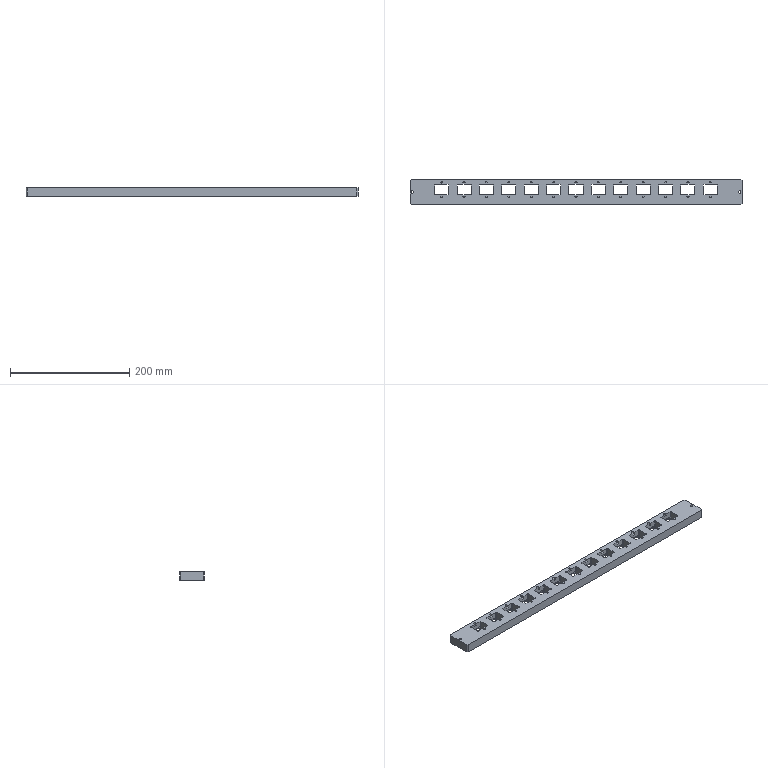NC program | NX | posted with a generic post | part box 556 x 41 x 15 mm
Lines 51164 to 52182 of 52182:
(PLANAR_MILL_COPY , TOOL : D6A45)
N102320 T07 M6
N102322 G54
N102324 G17 G0 G90 X-274.55 Y0.866 S7500 M3
N102326 G43 Z30. H7
N102328 Z1.8
N102330 G94 G1 Z-1.2 F1400.
N102332 G3 X-275.05 Y0. R1.
N102334 X-274. Y-1.05 R1.05
N102336 X-275.05 Y0. R-1.05
N102338 X-274.55 Y-0.866 R1.
N102340 G1 Z1.8
N102342 G0 Z30.
N102344 X-224.134 Y14.3
N102346 Z1.8
N102348 G1 Z-1.2
N102350 G3 X-225. Y14.8 R1.
N102352 G1 X-232.75
N102354 X-232.78 Y14.802
N102356 X-232.802 Y14.78
N102358 X-232.8 Y14.75
N102360 Y12.75
N102362 G2 X-233.75 Y11.8 R0.95
N102364 G1 X-235.75
N102366 X-235.78 Y11.802
N102368 X-235.802 Y11.78
N102370 X-235.8 Y11.75
N102372 Y-3.75
N102374 X-235.802 Y-3.78
N102376 X-235.78 Y-3.802
N102378 X-235.75 Y-3.8
N102380 X-233.75
N102382 G2 X-232.8 Y-4.75 R0.95
N102384 G1 Y-6.75
N102386 X-232.802 Y-6.78
N102388 X-232.78 Y-6.802
N102390 X-232.75 Y-6.8
N102392 X-217.25
N102394 X-217.22 Y-6.802
N102396 X-217.198 Y-6.78
N102398 X-217.2 Y-6.75
N102400 Y-4.75
N102402 G2 X-216.25 Y-3.8 R0.95
N102404 G1 X-214.25
N102406 X-214.22 Y-3.802
N102408 X-214.198 Y-3.78
N102410 X-214.2 Y-3.75
N102412 Y11.75
N102414 X-214.198 Y11.78
N102416 X-214.22 Y11.802
N102418 X-214.25 Y11.8
N102420 X-216.25
N102422 G2 X-217.2 Y12.75 R0.95
N102424 G1 Y14.75
N102426 X-217.198 Y14.78
N102428 X-217.22 Y14.802
N102430 X-217.25 Y14.8
N102432 X-225.
N102434 G3 X-225.866 Y14.3 R1.
N102436 G1 Z1.8
N102438 G0 Z30.
N102440 X-186.634
N102442 Z1.8
N102444 G1 Z-1.2
N102446 G3 X-187.5 Y14.8 R1.
N102448 G1 X-195.25
N102450 X-195.28 Y14.802
N102452 X-195.302 Y14.78
N102454 X-195.3 Y14.75
N102456 Y12.75
N102458 G2 X-196.25 Y11.8 R0.95
N102460 G1 X-198.25
N102462 X-198.28 Y11.802
N102464 X-198.302 Y11.78
N102466 X-198.3 Y11.75
N102468 Y-3.75
N102470 X-198.302 Y-3.78
N102472 X-198.28 Y-3.802
N102474 X-198.25 Y-3.8
N102476 X-196.25
N102478 G2 X-195.3 Y-4.75 R0.95
N102480 G1 Y-6.75
N102482 X-195.302 Y-6.78
N102484 X-195.28 Y-6.802
N102486 X-195.25 Y-6.8
N102488 X-179.75
N102490 X-179.72 Y-6.802
N102492 X-179.698 Y-6.78
N102494 X-179.7 Y-6.75
N102496 Y-4.75
N102498 G2 X-178.75 Y-3.8 R0.95
N102500 G1 X-176.75
N102502 X-176.72 Y-3.802
N102504 X-176.698 Y-3.78
N102506 X-176.7 Y-3.75
N102508 Y11.75
N102510 X-176.698 Y11.78
N102512 X-176.72 Y11.802
N102514 X-176.75 Y11.8
N102516 X-178.75
N102518 G2 X-179.7 Y12.75 R0.95
N102520 G1 Y14.75
N102522 X-179.698 Y14.78
N102524 X-179.72 Y14.802
N102526 X-179.75 Y14.8
N102528 X-187.5
N102530 G3 X-188.366 Y14.3 R1.
N102532 G1 Z1.8
N102534 G0 Z30.
N102536 X-149.134
N102538 Z1.8
N102540 G1 Z-1.2
N102542 G3 X-150. Y14.8 R1.
N102544 G1 X-157.75
N102546 X-157.78 Y14.802
N102548 X-157.802 Y14.78
N102550 X-157.8 Y14.75
N102552 Y12.75
N102554 G2 X-158.75 Y11.8 R0.95
N102556 G1 X-160.75
N102558 X-160.78 Y11.802
N102560 X-160.802 Y11.78
N102562 X-160.8 Y11.75
N102564 Y-3.75
N102566 X-160.802 Y-3.78
N102568 X-160.78 Y-3.802
N102570 X-160.75 Y-3.8
N102572 X-158.75
N102574 G2 X-157.8 Y-4.75 R0.95
N102576 G1 Y-6.75
N102578 X-157.802 Y-6.78
N102580 X-157.78 Y-6.802
N102582 X-157.75 Y-6.8
N102584 X-142.25
N102586 X-142.22 Y-6.802
N102588 X-142.198 Y-6.78
N102590 X-142.2 Y-6.75
N102592 Y-4.75
N102594 G2 X-141.25 Y-3.8 R0.95
N102596 G1 X-139.25
N102598 X-139.22 Y-3.802
N102600 X-139.198 Y-3.78
N102602 X-139.2 Y-3.75
N102604 Y11.75
N102606 X-139.198 Y11.78
N102608 X-139.22 Y11.802
N102610 X-139.25 Y11.8
N102612 X-141.25
N102614 G2 X-142.2 Y12.75 R0.95
N102616 G1 Y14.75
N102618 X-142.198 Y14.78
N102620 X-142.22 Y14.802
N102622 X-142.25 Y14.8
N102624 X-150.
N102626 G3 X-150.866 Y14.3 R1.
N102628 G1 Z1.8
N102630 G0 Z30.
N102632 X-111.634
N102634 Z1.8
N102636 G1 Z-1.2
N102638 G3 X-112.5 Y14.8 R1.
N102640 G1 X-120.25
N102642 X-120.28 Y14.802
N102644 X-120.302 Y14.78
N102646 X-120.3 Y14.75
N102648 Y12.75
N102650 G2 X-121.25 Y11.8 R0.95
N102652 G1 X-123.25
N102654 X-123.28 Y11.802
N102656 X-123.302 Y11.78
N102658 X-123.3 Y11.75
N102660 Y-3.75
N102662 X-123.302 Y-3.78
N102664 X-123.28 Y-3.802
N102666 X-123.25 Y-3.8
N102668 X-121.25
N102670 G2 X-120.3 Y-4.75 R0.95
N102672 G1 Y-6.75
N102674 X-120.302 Y-6.78
N102676 X-120.28 Y-6.802
N102678 X-120.25 Y-6.8
N102680 X-104.75
N102682 X-104.72 Y-6.802
N102684 X-104.698 Y-6.78
N102686 X-104.7 Y-6.75
N102688 Y-4.75
N102690 G2 X-103.75 Y-3.8 R0.95
N102692 G1 X-101.75
N102694 X-101.72 Y-3.802
N102696 X-101.698 Y-3.78
N102698 X-101.7 Y-3.75
N102700 Y11.75
N102702 X-101.698 Y11.78
N102704 X-101.72 Y11.802
N102706 X-101.75 Y11.8
N102708 X-103.75
N102710 G2 X-104.7 Y12.75 R0.95
N102712 G1 Y14.75
N102714 X-104.698 Y14.78
N102716 X-104.72 Y14.802
N102718 X-104.75 Y14.8
N102720 X-112.5
N102722 G3 X-113.366 Y14.3 R1.
N102724 G1 Z1.8
N102726 G0 Z30.
N102728 X-74.134
N102730 Z1.8
N102732 G1 Z-1.2
N102734 G3 X-75. Y14.8 R1.
N102736 G1 X-82.75
N102738 X-82.78 Y14.802
N102740 X-82.802 Y14.78
N102742 X-82.8 Y14.75
N102744 Y12.75
N102746 G2 X-83.75 Y11.8 R0.95
N102748 G1 X-85.75
N102750 X-85.78 Y11.802
N102752 X-85.802 Y11.78
N102754 X-85.8 Y11.75
N102756 Y-3.75
N102758 X-85.802 Y-3.78
N102760 X-85.78 Y-3.802
N102762 X-85.75 Y-3.8
N102764 X-83.75
N102766 G2 X-82.8 Y-4.75 R0.95
N102768 G1 Y-6.75
N102770 X-82.802 Y-6.78
N102772 X-82.78 Y-6.802
N102774 X-82.75 Y-6.8
N102776 X-67.25
N102778 X-67.22 Y-6.802
N102780 X-67.198 Y-6.78
N102782 X-67.2 Y-6.75
N102784 Y-4.75
N102786 G2 X-66.25 Y-3.8 R0.95
N102788 G1 X-64.25
N102790 X-64.22 Y-3.802
N102792 X-64.198 Y-3.78
N102794 X-64.2 Y-3.75
N102796 Y11.75
N102798 X-64.198 Y11.78
N102800 X-64.22 Y11.802
N102802 X-64.25 Y11.8
N102804 X-66.25
N102806 G2 X-67.2 Y12.75 R0.95
N102808 G1 Y14.75
N102810 X-67.198 Y14.78
N102812 X-67.22 Y14.802
N102814 X-67.25 Y14.8
N102816 X-75.
N102818 G3 X-75.866 Y14.3 R1.
N102820 G1 Z1.8
N102822 G0 Z30.
N102824 X-36.634
N102826 Z1.8
N102828 G1 Z-1.2
N102830 G3 X-37.5 Y14.8 R1.
N102832 G1 X-45.25
N102834 X-45.28 Y14.802
N102836 X-45.302 Y14.78
N102838 X-45.3 Y14.75
N102840 Y12.75
N102842 G2 X-46.25 Y11.8 R0.95
N102844 G1 X-48.25
N102846 X-48.28 Y11.802
N102848 X-48.302 Y11.78
N102850 X-48.3 Y11.75
N102852 Y-3.75
N102854 X-48.302 Y-3.78
N102856 X-48.28 Y-3.802
N102858 X-48.25 Y-3.8
N102860 X-46.25
N102862 G2 X-45.3 Y-4.75 R0.95
N102864 G1 Y-6.75
N102866 X-45.302 Y-6.78
N102868 X-45.28 Y-6.802
N102870 X-45.25 Y-6.8
N102872 X-29.75
N102874 X-29.72 Y-6.802
N102876 X-29.698 Y-6.78
N102878 X-29.7 Y-6.75
N102880 Y-4.75
N102882 G2 X-28.75 Y-3.8 R0.95
N102884 G1 X-26.75
N102886 X-26.72 Y-3.802
N102888 X-26.698 Y-3.78
N102890 X-26.7 Y-3.75
N102892 Y11.75
N102894 X-26.698 Y11.78
N102896 X-26.72 Y11.802
N102898 X-26.75 Y11.8
N102900 X-28.75
N102902 G2 X-29.7 Y12.75 R0.95
N102904 G1 Y14.75
N102906 X-29.698 Y14.78
N102908 X-29.72 Y14.802
N102910 X-29.75 Y14.8
N102912 X-37.5
N102914 G3 X-38.366 Y14.3 R1.
N102916 G1 Z1.8
N102918 G0 Z30.
N102920 X-0.866 Y21.95
N102922 Z1.8
N102924 G1 Z-1.2
N102926 G3 X0. Y21.45 R1.
N102928 G1 X276.
N102930 G2 X276.672 Y21.172 R0.95
N102932 G1 X278.672 Y19.172
N102934 G2 X278.95 Y18.5 R0.95
N102936 G1 Y-18.5
N102938 G2 X278.672 Y-19.172 R0.95
N102940 G1 X276.672 Y-21.172
N102942 G2 X276. Y-21.45 R0.95
N102944 G1 X-276.
N102946 G2 X-276.672 Y-21.172 R0.95
N102948 G1 X-278.672 Y-19.172
N102950 G2 X-278.95 Y-18.5 R0.95
N102952 G1 Y18.5
N102954 G2 X-278.672 Y19.172 R0.95
N102956 G1 X-276.672 Y21.172
N102958 G2 X-276. Y21.45 R0.95
N102960 G1 X0.
N102962 G3 X0.866 Y21.95 R1.
N102964 G1 Z1.8
N102966 G0 Z30.
N102968 Y14.3
N102970 Z1.8
N102972 G1 Z-1.2
N102974 G3 X0. Y14.8 R1.
N102976 G1 X-7.75
N102978 X-7.78 Y14.802
N102980 X-7.802 Y14.78
N102982 X-7.8 Y14.75
N102984 Y12.75
N102986 G2 X-8.75 Y11.8 R0.95
N102988 G1 X-10.75
N102990 X-10.78 Y11.802
N102992 X-10.802 Y11.78
N102994 X-10.8 Y11.75
N102996 Y-3.75
N102998 X-10.802 Y-3.78
N103000 X-10.78 Y-3.802
N103002 X-10.75 Y-3.8
N103004 X-8.75
N103006 G2 X-7.8 Y-4.75 R0.95
N103008 G1 Y-6.75
N103010 X-7.802 Y-6.78
N103012 X-7.78 Y-6.802
N103014 X-7.75 Y-6.8
N103016 X7.75
N103018 X7.78 Y-6.802
N103020 X7.802 Y-6.78
N103022 X7.8 Y-6.75
N103024 Y-4.75
N103026 G2 X8.75 Y-3.8 R0.95
N103028 G1 X10.75
N103030 X10.78 Y-3.802
N103032 X10.802 Y-3.78
N103034 X10.8 Y-3.75
N103036 Y11.75
N103038 X10.802 Y11.78
N103040 X10.78 Y11.802
N103042 X10.75 Y11.8
N103044 X8.75
N103046 G2 X7.8 Y12.75 R0.95
N103048 G1 Y14.75
N103050 X7.802 Y14.78
N103052 X7.78 Y14.802
N103054 X7.75 Y14.8
N103056 X0.
N103058 G3 X-0.866 Y14.3 R1.
N103060 G1 Z1.8
N103062 G0 Z30.
N103064 X38.366
N103066 Z1.8
N103068 G1 Z-1.2
N103070 G3 X37.5 Y14.8 R1.
N103072 G1 X29.75
N103074 X29.72 Y14.802
N103076 X29.698 Y14.78
N103078 X29.7 Y14.75
N103080 Y12.75
N103082 G2 X28.75 Y11.8 R0.95
N103084 G1 X26.75
N103086 X26.72 Y11.802
N103088 X26.698 Y11.78
N103090 X26.7 Y11.75
N103092 Y-3.75
N103094 X26.698 Y-3.78
N103096 X26.72 Y-3.802
N103098 X26.75 Y-3.8
N103100 X28.75
N103102 G2 X29.7 Y-4.75 R0.95
N103104 G1 Y-6.75
N103106 X29.698 Y-6.78
N103108 X29.72 Y-6.802
N103110 X29.75 Y-6.8
N103112 X45.25
N103114 X45.28 Y-6.802
N103116 X45.302 Y-6.78
N103118 X45.3 Y-6.75
N103120 Y-4.75
N103122 G2 X46.25 Y-3.8 R0.95
N103124 G1 X48.25
N103126 X48.28 Y-3.802
N103128 X48.302 Y-3.78
N103130 X48.3 Y-3.75
N103132 Y11.75
N103134 X48.302 Y11.78
N103136 X48.28 Y11.802
N103138 X48.25 Y11.8
N103140 X46.25
N103142 G2 X45.3 Y12.75 R0.95
N103144 G1 Y14.75
N103146 X45.302 Y14.78
N103148 X45.28 Y14.802
N103150 X45.25 Y14.8
N103152 X37.5
N103154 G3 X36.634 Y14.3 R1.
N103156 G1 Z1.8
N103158 G0 Z30.
N103160 X75.866
N103162 Z1.8
N103164 G1 Z-1.2
N103166 G3 X75. Y14.8 R1.
N103168 G1 X67.25
N103170 X67.22 Y14.802
N103172 X67.198 Y14.78
N103174 X67.2 Y14.75
N103176 Y12.75
N103178 G2 X66.25 Y11.8 R0.95
N103180 G1 X64.25
N103182 X64.22 Y11.802
N103184 X64.198 Y11.78
N103186 X64.2 Y11.75
N103188 Y-3.75
N103190 X64.198 Y-3.78
N103192 X64.22 Y-3.802
N103194 X64.25 Y-3.8
N103196 X66.25
N103198 G2 X67.2 Y-4.75 R0.95
N103200 G1 Y-6.75
N103202 X67.198 Y-6.78
N103204 X67.22 Y-6.802
N103206 X67.25 Y-6.8
N103208 X82.75
N103210 X82.78 Y-6.802
N103212 X82.802 Y-6.78
N103214 X82.8 Y-6.75
N103216 Y-4.75
N103218 G2 X83.75 Y-3.8 R0.95
N103220 G1 X85.75
N103222 X85.78 Y-3.802
N103224 X85.802 Y-3.78
N103226 X85.8 Y-3.75
N103228 Y11.75
N103230 X85.802 Y11.78
N103232 X85.78 Y11.802
N103234 X85.75 Y11.8
N103236 X83.75
N103238 G2 X82.8 Y12.75 R0.95
N103240 G1 Y14.75
N103242 X82.802 Y14.78
N103244 X82.78 Y14.802
N103246 X82.75 Y14.8
N103248 X75.
N103250 G3 X74.134 Y14.3 R1.
N103252 G1 Z1.8
N103254 G0 Z30.
N103256 X113.366
N103258 Z1.8
N103260 G1 Z-1.2
N103262 G3 X112.5 Y14.8 R1.
N103264 G1 X104.75
N103266 X104.72 Y14.802
N103268 X104.698 Y14.78
N103270 X104.7 Y14.75
N103272 Y12.75
N103274 G2 X103.75 Y11.8 R0.95
N103276 G1 X101.75
N103278 X101.72 Y11.802
N103280 X101.698 Y11.78
N103282 X101.7 Y11.75
N103284 Y-3.75
N103286 X101.698 Y-3.78
N103288 X101.72 Y-3.802
N103290 X101.75 Y-3.8
N103292 X103.75
N103294 G2 X104.7 Y-4.75 R0.95
N103296 G1 Y-6.75
N103298 X104.698 Y-6.78
N103300 X104.72 Y-6.802
N103302 X104.75 Y-6.8
N103304 X120.25
N103306 X120.28 Y-6.802
N103308 X120.302 Y-6.78
N103310 X120.3 Y-6.75
N103312 Y-4.75
N103314 G2 X121.25 Y-3.8 R0.95
N103316 G1 X123.25
N103318 X123.28 Y-3.802
N103320 X123.302 Y-3.78
N103322 X123.3 Y-3.75
N103324 Y11.75
N103326 X123.302 Y11.78
N103328 X123.28 Y11.802
N103330 X123.25 Y11.8
N103332 X121.25
N103334 G2 X120.3 Y12.75 R0.95
N103336 G1 Y14.75
N103338 X120.302 Y14.78
N103340 X120.28 Y14.802
N103342 X120.25 Y14.8
N103344 X112.5
N103346 G3 X111.634 Y14.3 R1.
N103348 G1 Z1.8
N103350 G0 Z30.
N103352 X150.866
N103354 Z1.8
N103356 G1 Z-1.2
N103358 G3 X150. Y14.8 R1.
N103360 G1 X142.25
N103362 X142.22 Y14.802
N103364 X142.198 Y14.78
N103366 X142.2 Y14.75
N103368 Y12.75
N103370 G2 X141.25 Y11.8 R0.95
N103372 G1 X139.25
N103374 X139.22 Y11.802
N103376 X139.198 Y11.78
N103378 X139.2 Y11.75
N103380 Y-3.75
N103382 X139.198 Y-3.78
N103384 X139.22 Y-3.802
N103386 X139.25 Y-3.8
N103388 X141.25
N103390 G2 X142.2 Y-4.75 R0.95
N103392 G1 Y-6.75
N103394 X142.198 Y-6.78
N103396 X142.22 Y-6.802
N103398 X142.25 Y-6.8
N103400 X157.75
N103402 X157.78 Y-6.802
N103404 X157.802 Y-6.78
N103406 X157.8 Y-6.75
N103408 Y-4.75
N103410 G2 X158.75 Y-3.8 R0.95
N103412 G1 X160.75
N103414 X160.78 Y-3.802
N103416 X160.802 Y-3.78
N103418 X160.8 Y-3.75
N103420 Y11.75
N103422 X160.802 Y11.78
N103424 X160.78 Y11.802
N103426 X160.75 Y11.8
N103428 X158.75
N103430 G2 X157.8 Y12.75 R0.95
N103432 G1 Y14.75
N103434 X157.802 Y14.78
N103436 X157.78 Y14.802
N103438 X157.75 Y14.8
N103440 X150.
N103442 G3 X149.134 Y14.3 R1.
N103444 G1 Z1.8
N103446 G0 Z30.
N103448 X188.366
N103450 Z1.8
N103452 G1 Z-1.2
N103454 G3 X187.5 Y14.8 R1.
N103456 G1 X179.75
N103458 X179.72 Y14.802
N103460 X179.698 Y14.78
N103462 X179.7 Y14.75
N103464 Y12.75
N103466 G2 X178.75 Y11.8 R0.95
N103468 G1 X176.75
N103470 X176.72 Y11.802
N103472 X176.698 Y11.78
N103474 X176.7 Y11.75
N103476 Y-3.75
N103478 X176.698 Y-3.78
N103480 X176.72 Y-3.802
N103482 X176.75 Y-3.8
N103484 X178.75
N103486 G2 X179.7 Y-4.75 R0.95
N103488 G1 Y-6.75
N103490 X179.698 Y-6.78
N103492 X179.72 Y-6.802
N103494 X179.75 Y-6.8
N103496 X195.25
N103498 X195.28 Y-6.802
N103500 X195.302 Y-6.78
N103502 X195.3 Y-6.75
N103504 Y-4.75
N103506 G2 X196.25 Y-3.8 R0.95
N103508 G1 X198.25
N103510 X198.28 Y-3.802
N103512 X198.302 Y-3.78
N103514 X198.3 Y-3.75
N103516 Y11.75
N103518 X198.302 Y11.78
N103520 X198.28 Y11.802
N103522 X198.25 Y11.8
N103524 X196.25
N103526 G2 X195.3 Y12.75 R0.95
N103528 G1 Y14.75
N103530 X195.302 Y14.78
N103532 X195.28 Y14.802
N103534 X195.25 Y14.8
N103536 X187.5
N103538 G3 X186.634 Y14.3 R1.
N103540 G1 Z1.8
N103542 G0 Z30.
N103544 X225.866
N103546 Z1.8
N103548 G1 Z-1.2
N103550 G3 X225. Y14.8 R1.
N103552 G1 X217.25
N103554 X217.22 Y14.802
N103556 X217.198 Y14.78
N103558 X217.2 Y14.75
N103560 Y12.75
N103562 G2 X216.25 Y11.8 R0.95
N103564 G1 X214.25
N103566 X214.22 Y11.802
N103568 X214.198 Y11.78
N103570 X214.2 Y11.75
N103572 Y-3.75
N103574 X214.198 Y-3.78
N103576 X214.22 Y-3.802
N103578 X214.25 Y-3.8
N103580 X216.25
N103582 G2 X217.2 Y-4.75 R0.95
N103584 G1 Y-6.75
N103586 X217.198 Y-6.78
N103588 X217.22 Y-6.802
N103590 X217.25 Y-6.8
N103592 X232.75
N103594 X232.78 Y-6.802
N103596 X232.802 Y-6.78
N103598 X232.8 Y-6.75
N103600 Y-4.75
N103602 G2 X233.75 Y-3.8 R0.95
N103604 G1 X235.75
N103606 X235.78 Y-3.802
N103608 X235.802 Y-3.78
N103610 X235.8 Y-3.75
N103612 Y11.75
N103614 X235.802 Y11.78
N103616 X235.78 Y11.802
N103618 X235.75 Y11.8
N103620 X233.75
N103622 G2 X232.8 Y12.75 R0.95
N103624 G1 Y14.75
N103626 X232.802 Y14.78
N103628 X232.78 Y14.802
N103630 X232.75 Y14.8
N103632 X225.
N103634 G3 X224.134 Y14.3 R1.
N103636 G1 Z1.8
N103638 G0 Z30.
N103640 X274.55 Y-0.866
N103642 Z1.8
N103644 G1 Z-1.2
N103646 G3 X275.05 Y0. R1.
N103648 X274. Y1.05 R1.05
N103650 X275.05 Y0. R-1.05
N103652 X274.55 Y0.866 R1.
N103654 G1 Z1.8
N103656 G0 Z30.
N103658 M5
(刀补_COPY , TOOL : D6JING)
N103660 T06 M6
N103662 G54
N103664 G17 G0 G90 X183.316 Y-3.49 S5000 M3
N103666 G43 Z30. H6
N103668 Z-4.
N103670 G94 G1 Z-5. F1000.
N103672 G41 X183.223 Y-3.525 D6
N103674 X182.071 Y-4.203
N103676 G3 X181.775 Y-4.725 R0.6
N103678 G1 X193.225
N103680 G3 X192.929 Y-4.203 R0.6
N103682 G1 X191.777 Y-3.525
N103684 G40
N103686 X191.684 Y-3.49
N103688 Z-4.
N103690 G0 Z30.
N103692 Y11.49
N103694 Z-4.
N103696 G1 Z-5.
N103698 G41 X191.777 Y11.525
N103700 X192.929 Y12.203
N103702 G3 X193.225 Y12.725 R0.6
N103704 G1 X181.775
N103706 G3 X182.071 Y12.203 R0.6
N103708 G1 X183.223 Y11.525
N103710 G40
N103712 X183.316 Y11.49
N103714 Z-4.
N103716 G0 Z30.
N103718 X145.816 Y-3.49
N103720 Z-4.
N103722 G1 Z-5.
N103724 G41 X145.723 Y-3.525
N103726 X144.571 Y-4.203
N103728 G3 X144.275 Y-4.725 R0.6
N103730 G1 X155.725
N103732 G3 X155.429 Y-4.203 R0.6
N103734 G1 X154.277 Y-3.525
N103736 G40
N103738 X154.184 Y-3.49
N103740 Z-4.
N103742 G0 Z30.
N103744 Y11.49
N103746 Z-4.
N103748 G1 Z-5.
N103750 G41 X154.277 Y11.525
N103752 X155.429 Y12.203
N103754 G3 X155.725 Y12.725 R0.6
N103756 G1 X144.275
N103758 G3 X144.571 Y12.203 R0.6
N103760 G1 X145.723 Y11.525
N103762 G40
N103764 X145.816 Y11.49
N103766 Z-4.
N103768 G0 Z30.
N103770 X108.316 Y-3.49
N103772 Z-4.
N103774 G1 Z-5.
N103776 G41 X108.223 Y-3.525
N103778 X107.071 Y-4.203
N103780 G3 X106.775 Y-4.725 R0.6
N103782 G1 X118.225
N103784 G3 X117.929 Y-4.203 R0.6
N103786 G1 X116.777 Y-3.525
N103788 G40
N103790 X116.684 Y-3.49
N103792 Z-4.
N103794 G0 Z30.
N103796 Y11.49
N103798 Z-4.
N103800 G1 Z-5.
N103802 G41 X116.777 Y11.525
N103804 X117.929 Y12.203
N103806 G3 X118.225 Y12.725 R0.6
N103808 G1 X106.775
N103810 G3 X107.071 Y12.203 R0.6
N103812 G1 X108.223 Y11.525
N103814 G40
N103816 X108.316 Y11.49
N103818 Z-4.
N103820 G0 Z30.
N103822 X70.816 Y-3.49
N103824 Z-4.
N103826 G1 Z-5.
N103828 G41 X70.723 Y-3.525
N103830 X69.571 Y-4.203
N103832 G3 X69.275 Y-4.725 R0.6
N103834 G1 X80.725
N103836 G3 X80.429 Y-4.203 R0.6
N103838 G1 X79.277 Y-3.525
N103840 G40
N103842 X79.184 Y-3.49
N103844 Z-4.
N103846 G0 Z30.
N103848 Y11.49
N103850 Z-4.
N103852 G1 Z-5.
N103854 G41 X79.277 Y11.525
N103856 X80.429 Y12.203
N103858 G3 X80.725 Y12.725 R0.6
N103860 G1 X69.275
N103862 G3 X69.571 Y12.203 R0.6
N103864 G1 X70.723 Y11.525
N103866 G40
N103868 X70.816 Y11.49
N103870 Z-4.
N103872 G0 Z30.
N103874 X33.316 Y-3.49
N103876 Z-4.
N103878 G1 Z-5.
N103880 G41 X33.223 Y-3.525
N103882 X32.071 Y-4.203
N103884 G3 X31.775 Y-4.725 R0.6
N103886 G1 X43.225
N103888 G3 X42.929 Y-4.203 R0.6
N103890 G1 X41.777 Y-3.525
N103892 G40
N103894 X41.684 Y-3.49
N103896 Z-4.
N103898 G0 Z30.
N103900 Y11.49
N103902 Z-4.
N103904 G1 Z-5.
N103906 G41 X41.777 Y11.525
N103908 X42.929 Y12.203
N103910 G3 X43.225 Y12.725 R0.6
N103912 G1 X31.775
N103914 G3 X32.071 Y12.203 R0.6
N103916 G1 X33.223 Y11.525
N103918 G40
N103920 X33.316 Y11.49
N103922 Z-4.
N103924 G0 Z30.
N103926 X-4.184 Y-3.49
N103928 Z-4.
N103930 G1 Z-5.
N103932 G41 X-4.277 Y-3.525
N103934 X-5.429 Y-4.203
N103936 G3 X-5.725 Y-4.725 R0.6
N103938 G1 X5.725
N103940 G3 X5.429 Y-4.203 R0.6
N103942 G1 X4.277 Y-3.525
N103944 G40
N103946 X4.184 Y-3.49
N103948 Z-4.
N103950 G0 Z30.
N103952 Y11.49
N103954 Z-4.
N103956 G1 Z-5.
N103958 G41 X4.277 Y11.525
N103960 X5.429 Y12.203
N103962 G3 X5.725 Y12.725 R0.6
N103964 G1 X-5.725
N103966 G3 X-5.429 Y12.203 R0.6
N103968 G1 X-4.277 Y11.525
N103970 G40
N103972 X-4.184 Y11.49
N103974 Z-4.
N103976 G0 Z30.
N103978 X-41.684 Y-3.49
N103980 Z-4.
N103982 G1 Z-5.
N103984 G41 X-41.777 Y-3.525
N103986 X-42.929 Y-4.203
N103988 G3 X-43.225 Y-4.725 R0.6
N103990 G1 X-31.775
N103992 G3 X-32.071 Y-4.203 R0.6
N103994 G1 X-33.223 Y-3.525
N103996 G40
N103998 X-33.316 Y-3.49
N104000 Z-4.
N104002 G0 Z30.
N104004 Y11.49
N104006 Z-4.
N104008 G1 Z-5.
N104010 G41 X-33.223 Y11.525
N104012 X-32.071 Y12.203
N104014 G3 X-31.775 Y12.725 R0.6
N104016 G1 X-43.225
N104018 G3 X-42.929 Y12.203 R0.6
N104020 G1 X-41.777 Y11.525
N104022 G40
N104024 X-41.684 Y11.49
N104026 Z-4.
N104028 G0 Z30.
N104030 X-79.184 Y-3.49
N104032 Z-4.
N104034 G1 Z-5.
N104036 G41 X-79.277 Y-3.525
N104038 X-80.429 Y-4.203
N104040 G3 X-80.725 Y-4.725 R0.6
N104042 G1 X-69.275
N104044 G3 X-69.571 Y-4.203 R0.6
N104046 G1 X-70.723 Y-3.525
N104048 G40
N104050 X-70.816 Y-3.49
N104052 Z-4.
N104054 G0 Z30.
N104056 Y11.49
N104058 Z-4.
N104060 G1 Z-5.
N104062 G41 X-70.723 Y11.525
N104064 X-69.571 Y12.203
N104066 G3 X-69.275 Y12.725 R0.6
N104068 G1 X-80.725
N104070 G3 X-80.429 Y12.203 R0.6
N104072 G1 X-79.277 Y11.525
N104074 G40
N104076 X-79.184 Y11.49
N104078 Z-4.
N104080 G0 Z30.
N104082 X-116.684 Y-3.49
N104084 Z-4.
N104086 G1 Z-5.
N104088 G41 X-116.777 Y-3.525
N104090 X-117.929 Y-4.203
N104092 G3 X-118.225 Y-4.725 R0.6
N104094 G1 X-106.775
N104096 G3 X-107.071 Y-4.203 R0.6
N104098 G1 X-108.223 Y-3.525
N104100 G40
N104102 X-108.316 Y-3.49
N104104 Z-4.
N104106 G0 Z30.
N104108 Y11.49
N104110 Z-4.
N104112 G1 Z-5.
N104114 G41 X-108.223 Y11.525
N104116 X-107.071 Y12.203
N104118 G3 X-106.775 Y12.725 R0.6
N104120 G1 X-118.225
N104122 G3 X-117.929 Y12.203 R0.6
N104124 G1 X-116.777 Y11.525
N104126 G40
N104128 X-116.684 Y11.49
N104130 Z-4.
N104132 G0 Z30.
N104134 X-154.184 Y-3.49
N104136 Z-4.
N104138 G1 Z-5.
N104140 G41 X-154.277 Y-3.525
N104142 X-155.429 Y-4.203
N104144 G3 X-155.725 Y-4.725 R0.6
N104146 G1 X-144.275
N104148 G3 X-144.571 Y-4.203 R0.6
N104150 G1 X-145.723 Y-3.525
N104152 G40
N104154 X-145.816 Y-3.49
N104156 Z-4.
N104158 G0 Z30.
N104160 Y11.49
N104162 Z-4.
N104164 G1 Z-5.
N104166 G41 X-145.723 Y11.525
N104168 X-144.571 Y12.203
N104170 G3 X-144.275 Y12.725 R0.6
N104172 G1 X-155.725
N104174 G3 X-155.429 Y12.203 R0.6
N104176 G1 X-154.277 Y11.525
N104178 G40
N104180 X-154.184 Y11.49
N104182 Z-4.
N104184 G0 Z30.
N104186 X-191.684 Y-3.49
N104188 Z-4.
N104190 G1 Z-5.
N104192 G41 X-191.777 Y-3.525
N104194 X-192.929 Y-4.203
N104196 G3 X-193.225 Y-4.725 R0.6
N104198 G1 X-181.775
N104200 G3 X-182.071 Y-4.203 R0.6
N104202 G1 X-183.223 Y-3.525
N104204 G40
N104206 X-183.316 Y-3.49
N104208 Z-4.
N104210 G0 Z30.
N104212 Y11.49
N104214 Z-4.
N104216 G1 Z-5.
N104218 G41 X-183.223 Y11.525
N104220 X-182.071 Y12.203
N104222 G3 X-181.775 Y12.725 R0.6
N104224 G1 X-193.225
N104226 G3 X-192.929 Y12.203 R0.6
N104228 G1 X-191.777 Y11.525
N104230 G40
N104232 X-191.684 Y11.49
N104234 Z-4.
N104236 G0 Z30.
N104238 X-229.184 Y-3.49
N104240 Z-4.
N104242 G1 Z-5.
N104244 G41 X-229.277 Y-3.525
N104246 X-230.429 Y-4.203
N104248 G3 X-230.725 Y-4.725 R0.6
N104250 G1 X-219.275
N104252 G3 X-219.571 Y-4.203 R0.6
N104254 G1 X-220.723 Y-3.525
N104256 G40
N104258 X-220.816 Y-3.49
N104260 Z-4.
N104262 G0 Z30.
N104264 Y11.49
N104266 Z-4.
N104268 G1 Z-5.
N104270 G41 X-220.723 Y11.525
N104272 X-219.571 Y12.203
N104274 G3 X-219.275 Y12.725 R0.6
N104276 G1 X-230.725
N104278 G3 X-230.429 Y12.203 R0.6
N104280 G1 X-229.277 Y11.525
N104282 G40
N104284 X-229.184 Y11.49
N104286 Z-4.
N104288 G0 Z30.
N104290 X220.816 Y-3.49
N104292 Z-4.
N104294 G1 Z-5.
N104296 G41 X220.723 Y-3.525
N104298 X219.571 Y-4.203
N104300 G3 X219.275 Y-4.725 R0.6
N104302 G1 X230.725
N104304 G3 X230.429 Y-4.203 R0.6
N104306 G1 X229.277 Y-3.525
N104308 G40
N104310 X229.184 Y-3.49
N104312 Z-4.
N104314 G0 Z30.
N104316 Y11.49
N104318 Z-4.
N104320 G1 Z-5.
N104322 G41 X229.277 Y11.525
N104324 X230.429 Y12.203
N104326 G3 X230.725 Y12.725 R0.6
N104328 G1 X219.275
N104330 G3 X219.571 Y12.203 R0.6
N104332 G1 X220.723 Y11.525
N104334 G40
N104336 X220.816 Y11.49
N104338 Z-4.
N104340 G0 Z30.
N104342 M5
N104344 M2